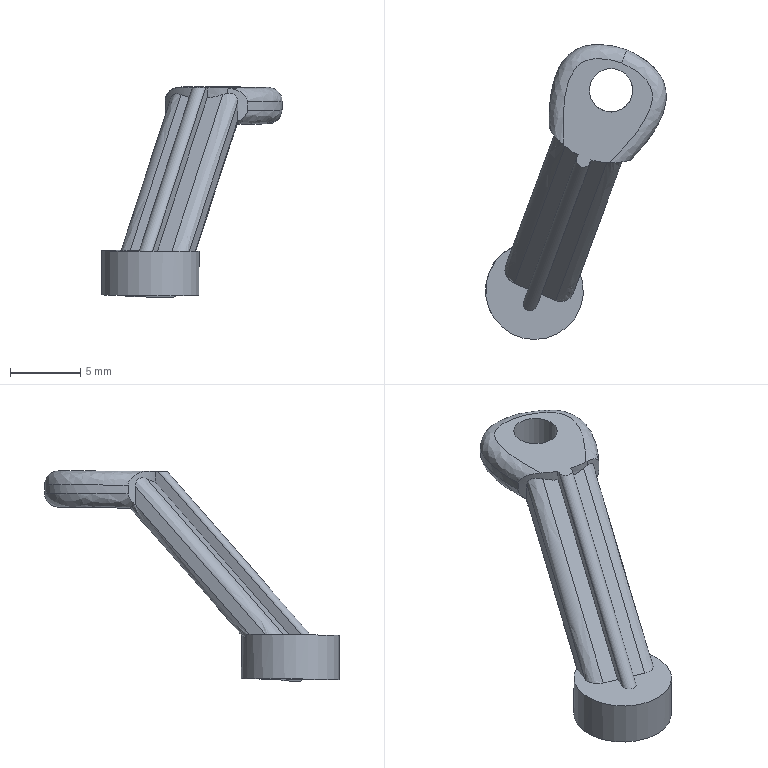Part | STEP file | 1 solid | 34 faces | box 12.902 x 21.037 x 15.015 mm | volume 400.583 mm3 | plane 15 | spline 14 | cylinder 5 | commonest cylinder face diameters 10.348 x3 3.1 x1 6.969 x1